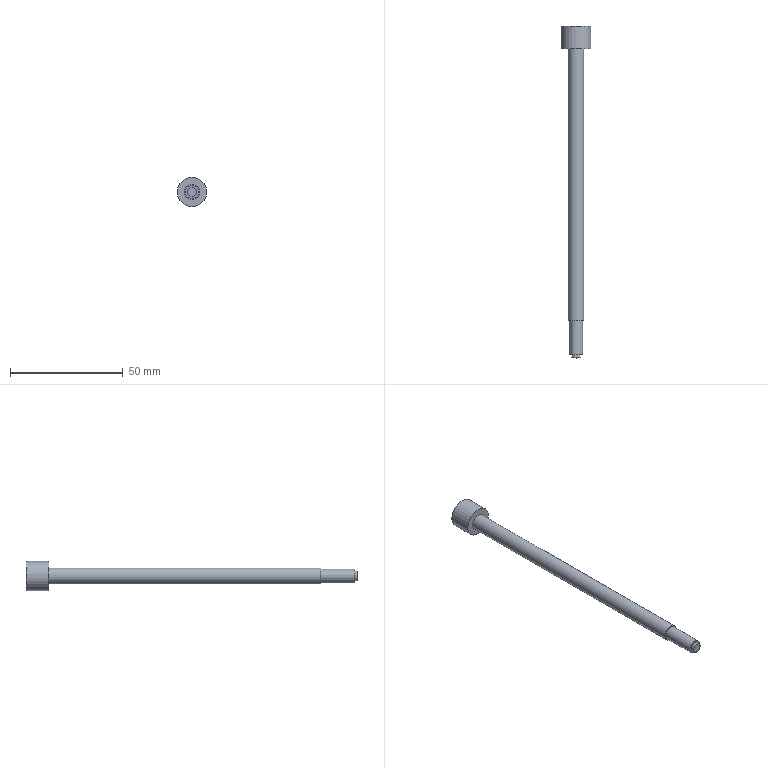Part | STEP file | solid 210 | 1 solid | 9 faces | box 13 x 147.06 x 13 mm | volume 6410 mm3 | plane 5 | cylinder 4 | commonest cylinder face diameters 4 x1 6 x1 7 x1 13 x1